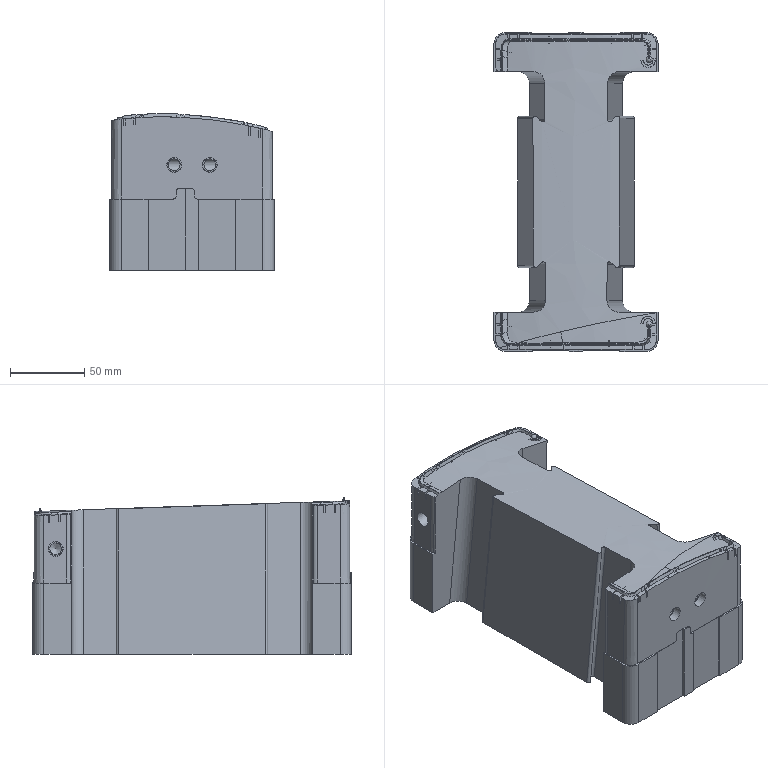Part | STEP file | P011002M002-000 | 2 solids | 754 faces | box 110.341 x 214.577 x 105.416 mm | volume 1490799 mm3 | plane 360 | spline 184 | cone 70 | other 69 | cylinder 69 | sphere 2 | commonest cylinder face diameters 8 x13 4.048 x10 3 x8 10.12 x8 10.2 x5 11.96 x5